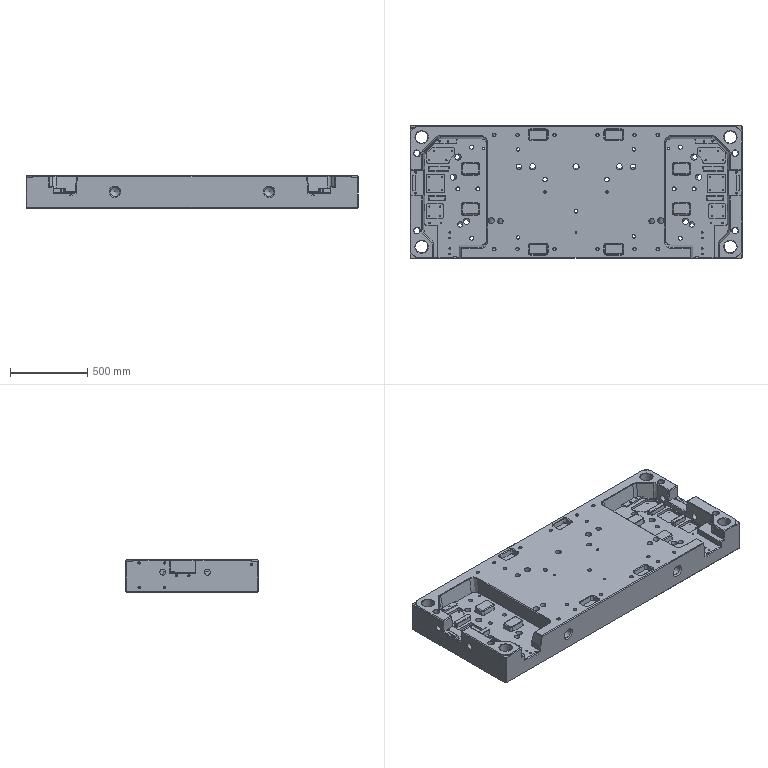Part | STEP file | solid 212 | 1 solid | 1240 faces | box 2150 x 860 x 210.001 mm | volume 305924028 mm3 | plane 341 | cylinder 340 | spline 278 | cone 276 | other 5 | commonest cylinder face diameters 26 x56 10.2 x48 13 x44 21 x32 6.8 x24 40 x23